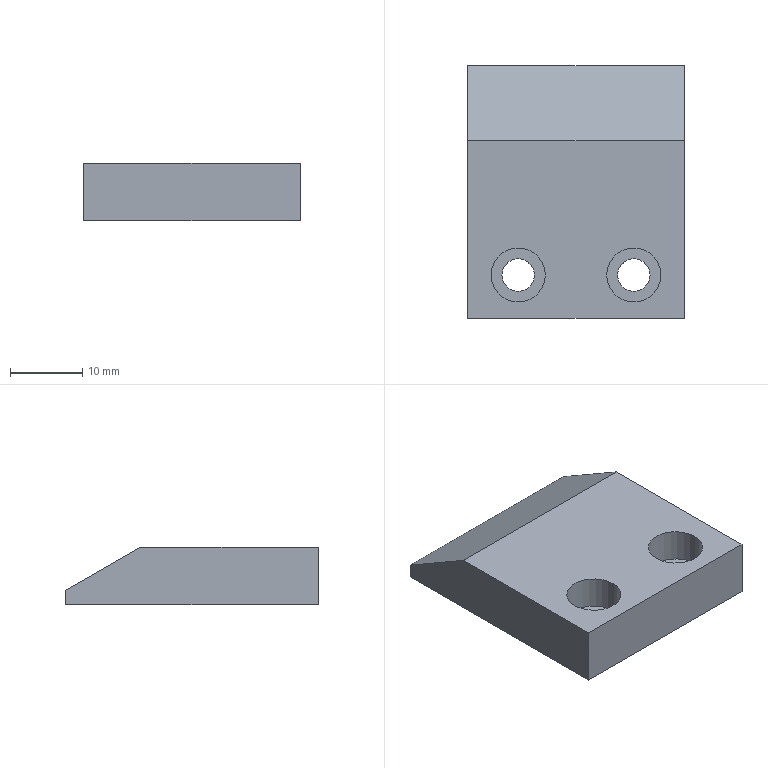Part | STEP file | BPSP-03-015 Shaft Pivot Seat | 1 solid | 17 faces | box 30 x 35 x 8 mm | volume 6950 mm3 | plane 9 | cylinder 8 | commonest cylinder face diameters 4.5 x4 7.5 x4
STEP:
#1=CARTESIAN_POINT('',(0.,0.,0.));
#2=DIRECTION('',(0.,0.,1.));
#3=DIRECTION('',(1.,0.,0.));
#4=AXIS2_PLACEMENT_3D('',#1,#2,#3);
#5=CARTESIAN_POINT('',(11.75,0.,-0.6));
#6=VERTEX_POINT('',#5);
#7=CARTESIAN_POINT('',(11.75,0.,4.));
#8=VERTEX_POINT('',#7);
#9=CARTESIAN_POINT('',(11.75,0.,4.));
#10=DIRECTION('',(0.,0.,1.));
#11=VECTOR('',#10,1.);
#12=LINE('',#9,#11);
#13=CARTESIAN_POINT('',(8.,0.,4.));
#14=DIRECTION('',(0.,0.,1.));
#15=DIRECTION('',(1.,0.,0.));
#16=AXIS2_PLACEMENT_3D('',#13,#14,#15);
#17=CYLINDRICAL_SURFACE('',#16,3.75);
#18=CARTESIAN_POINT('',(6.283,0.));
#19=DIRECTION('',(0.,1.));
#20=VECTOR('',#19,1.);
#21=LINE('',#18,#20);
#22=(GEOMETRIC_REPRESENTATION_CONTEXT(2)PARAMETRIC_REPRESENTATION_CONTEXT()REPRESENTATION_CONTEXT('',''));
#23=DEFINITIONAL_REPRESENTATION('',(#21),#22);
#24=PCURVE('',#17,#23);
#25=CARTESIAN_POINT('',(8.,0.,4.));
#26=DIRECTION('',(0.,0.,1.));
#27=DIRECTION('',(1.,0.,0.));
#28=AXIS2_PLACEMENT_3D('',#25,#26,#27);
#29=CYLINDRICAL_SURFACE('',#28,3.75);
#30=CARTESIAN_POINT('',(0.,0.));
#31=DIRECTION('',(0.,1.));
#32=VECTOR('',#31,1.);
#33=LINE('',#30,#32);
#34=(GEOMETRIC_REPRESENTATION_CONTEXT(2)PARAMETRIC_REPRESENTATION_CONTEXT()REPRESENTATION_CONTEXT('',''));
#35=DEFINITIONAL_REPRESENTATION('',(#33),#34);
#36=PCURVE('',#29,#35);
#37=SURFACE_CURVE('',#12,(#24,#36),.PCURVE_S1.);
#38=EDGE_CURVE('',#6,#8,#37,.T.);
#39=ORIENTED_EDGE('',*,*,#38,.T.);
#40=CARTESIAN_POINT('',(4.25,0.,4.));
#41=VERTEX_POINT('',#40);
#42=CARTESIAN_POINT('',(8.,0.,4.));
#43=DIRECTION('',(0.,0.,1.));
#44=DIRECTION('',(1.,0.,0.));
#45=AXIS2_PLACEMENT_3D('',#42,#43,#44);
#46=CIRCLE('',#45,3.75);
#47=CARTESIAN_POINT('',(0.,0.));
#48=DIRECTION('',(1.,0.));
#49=VECTOR('',#48,1.);
#50=LINE('',#47,#49);
#51=(GEOMETRIC_REPRESENTATION_CONTEXT(2)PARAMETRIC_REPRESENTATION_CONTEXT()REPRESENTATION_CONTEXT('',''));
#52=DEFINITIONAL_REPRESENTATION('',(#50),#51);
#53=PCURVE('',#17,#52);
#54=CARTESIAN_POINT('',(0.,0.,4.));
#55=DIRECTION('',(0.,0.,1.));
#56=DIRECTION('',(1.,0.,0.));
#57=AXIS2_PLACEMENT_3D('',#54,#55,#56);
#58=PLANE('',#57);
#59=CARTESIAN_POINT('',(8.,0.));
#60=DIRECTION('',(1.,0.));
#61=AXIS2_PLACEMENT_2D('',#59,#60);
#62=CIRCLE('',#61,3.75);
#63=(GEOMETRIC_REPRESENTATION_CONTEXT(2)PARAMETRIC_REPRESENTATION_CONTEXT()REPRESENTATION_CONTEXT('',''));
#64=DEFINITIONAL_REPRESENTATION('',(#62),#63);
#65=PCURVE('',#58,#64);
#66=SURFACE_CURVE('',#46,(#53,#65),.PCURVE_S1.);
#67=EDGE_CURVE('',#41,#8,#66,.T.);
#68=ORIENTED_EDGE('',*,*,#67,.F.);
#69=CARTESIAN_POINT('',(4.25,0.,-0.6));
#70=VERTEX_POINT('',#69);
#71=CARTESIAN_POINT('',(4.25,0.,4.));
#72=DIRECTION('',(0.,0.,1.));
#73=VECTOR('',#72,1.);
#74=LINE('',#71,#73);
#75=CARTESIAN_POINT('',(3.142,0.));
#76=DIRECTION('',(0.,1.));
#77=VECTOR('',#76,1.);
#78=LINE('',#75,#77);
#79=(GEOMETRIC_REPRESENTATION_CONTEXT(2)PARAMETRIC_REPRESENTATION_CONTEXT()REPRESENTATION_CONTEXT('',''));
#80=DEFINITIONAL_REPRESENTATION('',(#78),#79);
#81=PCURVE('',#17,#80);
#82=CARTESIAN_POINT('',(3.142,0.));
#83=DIRECTION('',(0.,1.));
#84=VECTOR('',#83,1.);
#85=LINE('',#82,#84);
#86=(GEOMETRIC_REPRESENTATION_CONTEXT(2)PARAMETRIC_REPRESENTATION_CONTEXT()REPRESENTATION_CONTEXT('',''));
#87=DEFINITIONAL_REPRESENTATION('',(#85),#86);
#88=PCURVE('',#29,#87);
#89=SURFACE_CURVE('',#74,(#81,#88),.PCURVE_S1.);
#90=EDGE_CURVE('',#70,#41,#89,.T.);
#91=ORIENTED_EDGE('',*,*,#90,.F.);
#92=CARTESIAN_POINT('',(8.,0.,-0.6));
#93=DIRECTION('',(0.,0.,1.));
#94=DIRECTION('',(1.,0.,0.));
#95=AXIS2_PLACEMENT_3D('',#92,#93,#94);
#96=CIRCLE('',#95,3.75);
#97=CARTESIAN_POINT('',(0.,-4.6));
#98=DIRECTION('',(1.,0.));
#99=VECTOR('',#98,1.);
#100=LINE('',#97,#99);
#101=(GEOMETRIC_REPRESENTATION_CONTEXT(2)PARAMETRIC_REPRESENTATION_CONTEXT()REPRESENTATION_CONTEXT('',''));
#102=DEFINITIONAL_REPRESENTATION('',(#100),#101);
#103=PCURVE('',#17,#102);
#104=CARTESIAN_POINT('',(10.25,0.,-0.6));
#105=DIRECTION('',(0.,0.,-1.));
#106=DIRECTION('',(-1.,0.,0.));
#107=AXIS2_PLACEMENT_3D('',#104,#105,#106);
#108=PLANE('',#107);
#109=CARTESIAN_POINT('',(-1.5,0.));
#110=CARTESIAN_POINT('',(-1.5,6.495));
#111=CARTESIAN_POINT('',(4.125,3.248));
#112=CARTESIAN_POINT('',(9.75,0.));
#113=CARTESIAN_POINT('',(4.125,-3.248));
#114=CARTESIAN_POINT('',(-1.5,-6.495));
#115=CARTESIAN_POINT('',(-1.5,0.));
#116=(BOUNDED_CURVE()B_SPLINE_CURVE(2,(#109,#110,#111,#112,#113,#114,#115),.UNSPECIFIED.,.T.,.F.)B_SPLINE_CURVE_WITH_KNOTS((1,2,2,2,2,1),(-2.094,0.,2.094,4.189,6.283,8.378),.UNSPECIFIED.)CURVE()GEOMETRIC_REPRESENTATION_ITEM()RATIONAL_B_SPLINE_CURVE((1.,0.5,1.,0.5,1.,0.5,1.))REPRESENTATION_ITEM(''));
#117=(GEOMETRIC_REPRESENTATION_CONTEXT(2)PARAMETRIC_REPRESENTATION_CONTEXT()REPRESENTATION_CONTEXT('',''));
#118=DEFINITIONAL_REPRESENTATION('',(#116),#117);
#119=PCURVE('',#108,#118);
#120=SURFACE_CURVE('',#96,(#103,#119),.PCURVE_S1.);
#121=EDGE_CURVE('',#70,#6,#120,.T.);
#122=ORIENTED_EDGE('',*,*,#121,.T.);
#123=EDGE_LOOP('',(#39,#68,#91,#122));
#124=FACE_BOUND('',#123,.F.);
#125=ADVANCED_FACE('',(#124),#17,.F.);
#126=CARTESIAN_POINT('',(10.25,0.,-4.));
#127=VERTEX_POINT('',#126);
#128=CARTESIAN_POINT('',(10.25,0.,-0.6));
#129=VERTEX_POINT('',#128);
#130=CARTESIAN_POINT('',(10.25,0.,4.));
#131=DIRECTION('',(0.,0.,1.));
#132=VECTOR('',#131,1.);
#133=LINE('',#130,#132);
#134=CARTESIAN_POINT('',(8.,0.,4.));
#135=DIRECTION('',(0.,0.,1.));
#136=DIRECTION('',(1.,0.,0.));
#137=AXIS2_PLACEMENT_3D('',#134,#135,#136);
#138=CYLINDRICAL_SURFACE('',#137,2.25);
#139=CARTESIAN_POINT('',(6.283,0.));
#140=DIRECTION('',(0.,1.));
#141=VECTOR('',#140,1.);
#142=LINE('',#139,#141);
#143=(GEOMETRIC_REPRESENTATION_CONTEXT(2)PARAMETRIC_REPRESENTATION_CONTEXT()REPRESENTATION_CONTEXT('',''));
#144=DEFINITIONAL_REPRESENTATION('',(#142),#143);
#145=PCURVE('',#138,#144);
#146=CARTESIAN_POINT('',(8.,0.,4.));
#147=DIRECTION('',(0.,0.,1.));
#148=DIRECTION('',(1.,0.,0.));
#149=AXIS2_PLACEMENT_3D('',#146,#147,#148);
#150=CYLINDRICAL_SURFACE('',#149,2.25);
#151=CARTESIAN_POINT('',(0.,0.));
#152=DIRECTION('',(0.,1.));
#153=VECTOR('',#152,1.);
#154=LINE('',#151,#153);
#155=(GEOMETRIC_REPRESENTATION_CONTEXT(2)PARAMETRIC_REPRESENTATION_CONTEXT()REPRESENTATION_CONTEXT('',''));
#156=DEFINITIONAL_REPRESENTATION('',(#154),#155);
#157=PCURVE('',#150,#156);
#158=SURFACE_CURVE('',#133,(#145,#157),.PCURVE_S1.);
#159=EDGE_CURVE('',#127,#129,#158,.T.);
#160=ORIENTED_EDGE('',*,*,#159,.T.);
#161=CARTESIAN_POINT('',(5.75,0.,-0.6));
#162=VERTEX_POINT('',#161);
#163=CARTESIAN_POINT('',(8.,0.,-0.6));
#164=DIRECTION('',(0.,0.,1.));
#165=DIRECTION('',(1.,0.,0.));
#166=AXIS2_PLACEMENT_3D('',#163,#164,#165);
#167=CIRCLE('',#166,2.25);
#168=CARTESIAN_POINT('',(0.,-4.6));
#169=DIRECTION('',(1.,0.));
#170=VECTOR('',#169,1.);
#171=LINE('',#168,#170);
#172=(GEOMETRIC_REPRESENTATION_CONTEXT(2)PARAMETRIC_REPRESENTATION_CONTEXT()REPRESENTATION_CONTEXT('',''));
#173=DEFINITIONAL_REPRESENTATION('',(#171),#172);
#174=PCURVE('',#138,#173);
#175=CARTESIAN_POINT('',(0.,0.));
#176=CARTESIAN_POINT('',(0.,3.897));
#177=CARTESIAN_POINT('',(3.375,1.949));
#178=CARTESIAN_POINT('',(6.75,0.));
#179=CARTESIAN_POINT('',(3.375,-1.949));
#180=CARTESIAN_POINT('',(0.,-3.897));
#181=CARTESIAN_POINT('',(0.,0.));
#182=(BOUNDED_CURVE()B_SPLINE_CURVE(2,(#175,#176,#177,#178,#179,#180,#181),.UNSPECIFIED.,.T.,.F.)B_SPLINE_CURVE_WITH_KNOTS((1,2,2,2,2,1),(-2.094,0.,2.094,4.189,6.283,8.378),.UNSPECIFIED.)CURVE()GEOMETRIC_REPRESENTATION_ITEM()RATIONAL_B_SPLINE_CURVE((1.,0.5,1.,0.5,1.,0.5,1.))REPRESENTATION_ITEM(''));
#183=(GEOMETRIC_REPRESENTATION_CONTEXT(2)PARAMETRIC_REPRESENTATION_CONTEXT()REPRESENTATION_CONTEXT('',''));
#184=DEFINITIONAL_REPRESENTATION('',(#182),#183);
#185=PCURVE('',#108,#184);
#186=SURFACE_CURVE('',#167,(#174,#185),.PCURVE_S1.);
#187=EDGE_CURVE('',#162,#129,#186,.T.);
#188=ORIENTED_EDGE('',*,*,#187,.F.);
#189=CARTESIAN_POINT('',(5.75,0.,-4.));
#190=VERTEX_POINT('',#189);
#191=CARTESIAN_POINT('',(5.75,0.,4.));
#192=DIRECTION('',(0.,0.,1.));
#193=VECTOR('',#192,1.);
#194=LINE('',#191,#193);
#195=CARTESIAN_POINT('',(3.142,0.));
#196=DIRECTION('',(0.,1.));
#197=VECTOR('',#196,1.);
#198=LINE('',#195,#197);
#199=(GEOMETRIC_REPRESENTATION_CONTEXT(2)PARAMETRIC_REPRESENTATION_CONTEXT()REPRESENTATION_CONTEXT('',''));
#200=DEFINITIONAL_REPRESENTATION('',(#198),#199);
#201=PCURVE('',#138,#200);
#202=CARTESIAN_POINT('',(3.142,0.));
#203=DIRECTION('',(0.,1.));
#204=VECTOR('',#203,1.);
#205=LINE('',#202,#204);
#206=(GEOMETRIC_REPRESENTATION_CONTEXT(2)PARAMETRIC_REPRESENTATION_CONTEXT()REPRESENTATION_CONTEXT('',''));
#207=DEFINITIONAL_REPRESENTATION('',(#205),#206);
#208=PCURVE('',#150,#207);
#209=SURFACE_CURVE('',#194,(#201,#208),.PCURVE_S1.);
#210=EDGE_CURVE('',#190,#162,#209,.T.);
#211=ORIENTED_EDGE('',*,*,#210,.F.);
#212=CARTESIAN_POINT('',(8.,0.,-4.));
#213=DIRECTION('',(0.,0.,1.));
#214=DIRECTION('',(1.,0.,0.));
#215=AXIS2_PLACEMENT_3D('',#212,#213,#214);
#216=CIRCLE('',#215,2.25);
#217=CARTESIAN_POINT('',(0.,-8.));
#218=DIRECTION('',(1.,0.));
#219=VECTOR('',#218,1.);
#220=LINE('',#217,#219);
#221=(GEOMETRIC_REPRESENTATION_CONTEXT(2)PARAMETRIC_REPRESENTATION_CONTEXT()REPRESENTATION_CONTEXT('',''));
#222=DEFINITIONAL_REPRESENTATION('',(#220),#221);
#223=PCURVE('',#138,#222);
#224=CARTESIAN_POINT('',(0.,0.,-4.));
#225=DIRECTION('',(0.,0.,1.));
#226=DIRECTION('',(1.,0.,0.));
#227=AXIS2_PLACEMENT_3D('',#224,#225,#226);
#228=PLANE('',#227);
#229=CARTESIAN_POINT('',(8.,0.));
#230=DIRECTION('',(1.,0.));
#231=AXIS2_PLACEMENT_2D('',#229,#230);
#232=CIRCLE('',#231,2.25);
#233=(GEOMETRIC_REPRESENTATION_CONTEXT(2)PARAMETRIC_REPRESENTATION_CONTEXT()REPRESENTATION_CONTEXT('',''));
#234=DEFINITIONAL_REPRESENTATION('',(#232),#233);
#235=PCURVE('',#228,#234);
#236=SURFACE_CURVE('',#216,(#223,#235),.PCURVE_S1.);
#237=EDGE_CURVE('',#190,#127,#236,.T.);
#238=ORIENTED_EDGE('',*,*,#237,.T.);
#239=EDGE_LOOP('',(#160,#188,#211,#238));
#240=FACE_BOUND('',#239,.F.);
#241=ADVANCED_FACE('',(#240),#138,.F.);
#242=CARTESIAN_POINT('',(-4.25,0.,-0.6));
#243=VERTEX_POINT('',#242);
#244=CARTESIAN_POINT('',(-4.25,0.,4.));
#245=VERTEX_POINT('',#244);
#246=CARTESIAN_POINT('',(-4.25,0.,4.));
#247=DIRECTION('',(0.,0.,1.));
#248=VECTOR('',#247,1.);
#249=LINE('',#246,#248);
#250=CARTESIAN_POINT('',(-8.,0.,4.));
#251=DIRECTION('',(0.,0.,1.));
#252=DIRECTION('',(1.,0.,0.));
#253=AXIS2_PLACEMENT_3D('',#250,#251,#252);
#254=CYLINDRICAL_SURFACE('',#253,3.75);
#255=CARTESIAN_POINT('',(6.283,0.));
#256=DIRECTION('',(0.,1.));
#257=VECTOR('',#256,1.);
#258=LINE('',#255,#257);
#259=(GEOMETRIC_REPRESENTATION_CONTEXT(2)PARAMETRIC_REPRESENTATION_CONTEXT()REPRESENTATION_CONTEXT('',''));
#260=DEFINITIONAL_REPRESENTATION('',(#258),#259);
#261=PCURVE('',#254,#260);
#262=CARTESIAN_POINT('',(-8.,0.,4.));
#263=DIRECTION('',(0.,0.,1.));
#264=DIRECTION('',(1.,0.,0.));
#265=AXIS2_PLACEMENT_3D('',#262,#263,#264);
#266=CYLINDRICAL_SURFACE('',#265,3.75);
#267=CARTESIAN_POINT('',(0.,0.));
#268=DIRECTION('',(0.,1.));
#269=VECTOR('',#268,1.);
#270=LINE('',#267,#269);
#271=(GEOMETRIC_REPRESENTATION_CONTEXT(2)PARAMETRIC_REPRESENTATION_CONTEXT()REPRESENTATION_CONTEXT('',''));
#272=DEFINITIONAL_REPRESENTATION('',(#270),#271);
#273=PCURVE('',#266,#272);
#274=SURFACE_CURVE('',#249,(#261,#273),.PCURVE_S1.);
#275=EDGE_CURVE('',#243,#245,#274,.T.);
#276=ORIENTED_EDGE('',*,*,#275,.T.);
#277=CARTESIAN_POINT('',(-11.75,0.,4.));
#278=VERTEX_POINT('',#277);
#279=CARTESIAN_POINT('',(-8.,0.,4.));
#280=DIRECTION('',(0.,0.,1.));
#281=DIRECTION('',(1.,0.,0.));
#282=AXIS2_PLACEMENT_3D('',#279,#280,#281);
#283=CIRCLE('',#282,3.75);
#284=CARTESIAN_POINT('',(0.,0.));
#285=DIRECTION('',(1.,0.));
#286=VECTOR('',#285,1.);
#287=LINE('',#284,#286);
#288=(GEOMETRIC_REPRESENTATION_CONTEXT(2)PARAMETRIC_REPRESENTATION_CONTEXT()REPRESENTATION_CONTEXT('',''));
#289=DEFINITIONAL_REPRESENTATION('',(#287),#288);
#290=PCURVE('',#254,#289);
#291=CARTESIAN_POINT('',(-8.,0.));
#292=DIRECTION('',(1.,0.));
#293=AXIS2_PLACEMENT_2D('',#291,#292);
#294=CIRCLE('',#293,3.75);
#295=(GEOMETRIC_REPRESENTATION_CONTEXT(2)PARAMETRIC_REPRESENTATION_CONTEXT()REPRESENTATION_CONTEXT('',''));
#296=DEFINITIONAL_REPRESENTATION('',(#294),#295);
#297=PCURVE('',#58,#296);
#298=SURFACE_CURVE('',#283,(#290,#297),.PCURVE_S1.);
#299=EDGE_CURVE('',#278,#245,#298,.T.);
#300=ORIENTED_EDGE('',*,*,#299,.F.);
#301=CARTESIAN_POINT('',(-11.75,0.,-0.6));
#302=VERTEX_POINT('',#301);
#303=CARTESIAN_POINT('',(-11.75,0.,4.));
#304=DIRECTION('',(0.,0.,1.));
#305=VECTOR('',#304,1.);
#306=LINE('',#303,#305);
#307=CARTESIAN_POINT('',(3.142,0.));
#308=DIRECTION('',(0.,1.));
#309=VECTOR('',#308,1.);
#310=LINE('',#307,#309);
#311=(GEOMETRIC_REPRESENTATION_CONTEXT(2)PARAMETRIC_REPRESENTATION_CONTEXT()REPRESENTATION_CONTEXT('',''));
#312=DEFINITIONAL_REPRESENTATION('',(#310),#311);
#313=PCURVE('',#254,#312);
#314=CARTESIAN_POINT('',(3.142,0.));
#315=DIRECTION('',(0.,1.));
#316=VECTOR('',#315,1.);
#317=LINE('',#314,#316);
#318=(GEOMETRIC_REPRESENTATION_CONTEXT(2)PARAMETRIC_REPRESENTATION_CONTEXT()REPRESENTATION_CONTEXT('',''));
#319=DEFINITIONAL_REPRESENTATION('',(#317),#318);
#320=PCURVE('',#266,#319);
#321=SURFACE_CURVE('',#306,(#313,#320),.PCURVE_S1.);
#322=EDGE_CURVE('',#302,#278,#321,.T.);
#323=ORIENTED_EDGE('',*,*,#322,.F.);
#324=CARTESIAN_POINT('',(-8.,0.,-0.6));
#325=DIRECTION('',(0.,0.,1.));
#326=DIRECTION('',(1.,0.,0.));
#327=AXIS2_PLACEMENT_3D('',#324,#325,#326);
#328=CIRCLE('',#327,3.75);
#329=CARTESIAN_POINT('',(0.,-4.6));
#330=DIRECTION('',(1.,0.));
#331=VECTOR('',#330,1.);
#332=LINE('',#329,#331);
#333=(GEOMETRIC_REPRESENTATION_CONTEXT(2)PARAMETRIC_REPRESENTATION_CONTEXT()REPRESENTATION_CONTEXT('',''));
#334=DEFINITIONAL_REPRESENTATION('',(#332),#333);
#335=PCURVE('',#254,#334);
#336=CARTESIAN_POINT('',(-5.75,0.,-0.6));
#337=DIRECTION('',(0.,0.,-1.));
#338=DIRECTION('',(-1.,0.,0.));
#339=AXIS2_PLACEMENT_3D('',#336,#337,#338);
#340=PLANE('',#339);
#341=CARTESIAN_POINT('',(-1.5,0.));
#342=CARTESIAN_POINT('',(-1.5,6.495));
#343=CARTESIAN_POINT('',(4.125,3.248));
#344=CARTESIAN_POINT('',(9.75,0.));
#345=CARTESIAN_POINT('',(4.125,-3.248));
#346=CARTESIAN_POINT('',(-1.5,-6.495));
#347=CARTESIAN_POINT('',(-1.5,0.));
#348=(BOUNDED_CURVE()B_SPLINE_CURVE(2,(#341,#342,#343,#344,#345,#346,#347),.UNSPECIFIED.,.T.,.F.)B_SPLINE_CURVE_WITH_KNOTS((1,2,2,2,2,1),(-2.094,0.,2.094,4.189,6.283,8.378),.UNSPECIFIED.)CURVE()GEOMETRIC_REPRESENTATION_ITEM()RATIONAL_B_SPLINE_CURVE((1.,0.5,1.,0.5,1.,0.5,1.))REPRESENTATION_ITEM(''));
#349=(GEOMETRIC_REPRESENTATION_CONTEXT(2)PARAMETRIC_REPRESENTATION_CONTEXT()REPRESENTATION_CONTEXT('',''));
#350=DEFINITIONAL_REPRESENTATION('',(#348),#349);
#351=PCURVE('',#340,#350);
#352=SURFACE_CURVE('',#328,(#335,#351),.PCURVE_S1.);
#353=EDGE_CURVE('',#302,#243,#352,.T.);
#354=ORIENTED_EDGE('',*,*,#353,.T.);
#355=EDGE_LOOP('',(#276,#300,#323,#354));
#356=FACE_BOUND('',#355,.F.);
#357=ADVANCED_FACE('',(#356),#254,.F.);
#358=CARTESIAN_POINT('',(-5.75,0.,-4.));
#359=VERTEX_POINT('',#358);
#360=CARTESIAN_POINT('',(-5.75,0.,-0.6));
#361=VERTEX_POINT('',#360);
#362=CARTESIAN_POINT('',(-5.75,0.,4.));
#363=DIRECTION('',(0.,0.,1.));
#364=VECTOR('',#363,1.);
#365=LINE('',#362,#364);
#366=CARTESIAN_POINT('',(-8.,0.,4.));
#367=DIRECTION('',(0.,0.,1.));
#368=DIRECTION('',(1.,0.,0.));
#369=AXIS2_PLACEMENT_3D('',#366,#367,#368);
#370=CYLINDRICAL_SURFACE('',#369,2.25);
#371=CARTESIAN_POINT('',(6.283,0.));
#372=DIRECTION('',(0.,1.));
#373=VECTOR('',#372,1.);
#374=LINE('',#371,#373);
#375=(GEOMETRIC_REPRESENTATION_CONTEXT(2)PARAMETRIC_REPRESENTATION_CONTEXT()REPRESENTATION_CONTEXT('',''));
#376=DEFINITIONAL_REPRESENTATION('',(#374),#375);
#377=PCURVE('',#370,#376);
#378=CARTESIAN_POINT('',(-8.,0.,4.));
#379=DIRECTION('',(0.,0.,1.));
#380=DIRECTION('',(1.,0.,0.));
#381=AXIS2_PLACEMENT_3D('',#378,#379,#380);
#382=CYLINDRICAL_SURFACE('',#381,2.25);
#383=CARTESIAN_POINT('',(0.,0.));
#384=DIRECTION('',(0.,1.));
#385=VECTOR('',#384,1.);
#386=LINE('',#383,#385);
#387=(GEOMETRIC_REPRESENTATION_CONTEXT(2)PARAMETRIC_REPRESENTATION_CONTEXT()REPRESENTATION_CONTEXT('',''));
#388=DEFINITIONAL_REPRESENTATION('',(#386),#387);
#389=PCURVE('',#382,#388);
#390=SURFACE_CURVE('',#365,(#377,#389),.PCURVE_S1.);
#391=EDGE_CURVE('',#359,#361,#390,.T.);
#392=ORIENTED_EDGE('',*,*,#391,.T.);
#393=CARTESIAN_POINT('',(-10.25,0.,-0.6));
#394=VERTEX_POINT('',#393);
#395=CARTESIAN_POINT('',(-8.,0.,-0.6));
#396=DIRECTION('',(0.,0.,1.));
#397=DIRECTION('',(1.,0.,0.));
#398=AXIS2_PLACEMENT_3D('',#395,#396,#397);
#399=CIRCLE('',#398,2.25);
#400=CARTESIAN_POINT('',(0.,-4.6));
#401=DIRECTION('',(1.,0.));
#402=VECTOR('',#401,1.);
#403=LINE('',#400,#402);
#404=(GEOMETRIC_REPRESENTATION_CONTEXT(2)PARAMETRIC_REPRESENTATION_CONTEXT()REPRESENTATION_CONTEXT('',''));
#405=DEFINITIONAL_REPRESENTATION('',(#403),#404);
#406=PCURVE('',#370,#405);
#407=CARTESIAN_POINT('',(0.,0.));
#408=CARTESIAN_POINT('',(0.,3.897));
#409=CARTESIAN_POINT('',(3.375,1.949));
#410=CARTESIAN_POINT('',(6.75,0.));
#411=CARTESIAN_POINT('',(3.375,-1.949));
#412=CARTESIAN_POINT('',(0.,-3.897));
#413=CARTESIAN_POINT('',(0.,0.));
#414=(BOUNDED_CURVE()B_SPLINE_CURVE(2,(#407,#408,#409,#410,#411,#412,#413),.UNSPECIFIED.,.T.,.F.)B_SPLINE_CURVE_WITH_KNOTS((1,2,2,2,2,1),(-2.094,0.,2.094,4.189,6.283,8.378),.UNSPECIFIED.)CURVE()GEOMETRIC_REPRESENTATION_ITEM()RATIONAL_B_SPLINE_CURVE((1.,0.5,1.,0.5,1.,0.5,1.))REPRESENTATION_ITEM(''));
#415=(GEOMETRIC_REPRESENTATION_CONTEXT(2)PARAMETRIC_REPRESENTATION_CONTEXT()REPRESENTATION_CONTEXT('',''));
#416=DEFINITIONAL_REPRESENTATION('',(#414),#415);
#417=PCURVE('',#340,#416);
#418=SURFACE_CURVE('',#399,(#406,#417),.PCURVE_S1.);
#419=EDGE_CURVE('',#394,#361,#418,.T.);
#420=ORIENTED_EDGE('',*,*,#419,.F.);
#421=CARTESIAN_POINT('',(-10.25,0.,-4.));
#422=VERTEX_POINT('',#421);
#423=CARTESIAN_POINT('',(-10.25,0.,4.));
#424=DIRECTION('',(0.,0.,1.));
#425=VECTOR('',#424,1.);
#426=LINE('',#423,#425);
#427=CARTESIAN_POINT('',(3.142,0.));
#428=DIRECTION('',(0.,1.));
#429=VECTOR('',#428,1.);
#430=LINE('',#427,#429);
#431=(GEOMETRIC_REPRESENTATION_CONTEXT(2)PARAMETRIC_REPRESENTATION_CONTEXT()REPRESENTATION_CONTEXT('',''));
#432=DEFINITIONAL_REPRESENTATION('',(#430),#431);
#433=PCURVE('',#370,#432);
#434=CARTESIAN_POINT('',(3.142,0.));
#435=DIRECTION('',(0.,1.));
#436=VECTOR('',#435,1.);
#437=LINE('',#434,#436);
#438=(GEOMETRIC_REPRESENTATION_CONTEXT(2)PARAMETRIC_REPRESENTATION_CONTEXT()REPRESENTATION_CONTEXT('',''));
#439=DEFINITIONAL_REPRESENTATION('',(#437),#438);
#440=PCURVE('',#382,#439);
#441=SURFACE_CURVE('',#426,(#433,#440),.PCURVE_S1.);
#442=EDGE_CURVE('',#422,#394,#441,.T.);
#443=ORIENTED_EDGE('',*,*,#442,.F.);
#444=CARTESIAN_POINT('',(-8.,0.,-4.));
#445=DIRECTION('',(0.,0.,1.));
#446=DIRECTION('',(1.,0.,0.));
#447=AXIS2_PLACEMENT_3D('',#444,#445,#446);
#448=CIRCLE('',#447,2.25);
#449=CARTESIAN_POINT('',(0.,-8.));
#450=DIRECTION('',(1.,0.));
#451=VECTOR('',#450,1.);
#452=LINE('',#449,#451);
#453=(GEOMETRIC_REPRESENTATION_CONTEXT(2)PARAMETRIC_REPRESENTATION_CONTEXT()REPRESENTATION_CONTEXT('',''));
#454=DEFINITIONAL_REPRESENTATION('',(#452),#453);
#455=PCURVE('',#370,#454);
#456=CARTESIAN_POINT('',(-8.,0.));
#457=DIRECTION('',(1.,0.));
#458=AXIS2_PLACEMENT_2D('',#456,#457);
#459=CIRCLE('',#458,2.25);
#460=(GEOMETRIC_REPRESENTATION_CONTEXT(2)PARAMETRIC_REPRESENTATION_CONTEXT()REPRESENTATION_CONTEXT('',''));
#461=DEFINITIONAL_REPRESENTATION('',(#459),#460);
#462=PCURVE('',#228,#461);
#463=SURFACE_CURVE('',#448,(#455,#462),.PCURVE_S1.);
#464=EDGE_CURVE('',#422,#359,#463,.T.);
#465=ORIENTED_EDGE('',*,*,#464,.T.);
#466=EDGE_LOOP('',(#392,#420,#443,#465));
#467=FACE_BOUND('',#466,.F.);
#468=ADVANCED_FACE('',(#467),#370,.F.);
#469=CARTESIAN_POINT('',(-15.,18.608,4.));
#470=VERTEX_POINT('',#469);
#471=CARTESIAN_POINT('',(-15.,-6.,4.));
#472=VERTEX_POINT('',#471);
#473=CARTESIAN_POINT('',(-15.,29.,4.));
#474=DIRECTION('',(0.,-1.,0.));
#475=VECTOR('',#474,1.);
#476=LINE('',#473,#475);
#477=CARTESIAN_POINT('',(-15.,29.,4.));
#478=DIRECTION('',(1.,0.,0.));
#479=DIRECTION('',(0.,1.,0.));
#480=AXIS2_PLACEMENT_3D('',#477,#478,#479);
#481=PLANE('',#480);
#482=CARTESIAN_POINT('',(0.,0.));
#483=DIRECTION('',(-1.,0.));
#484=VECTOR('',#483,1.);
#485=LINE('',#482,#484);
#486=(GEOMETRIC_REPRESENTATION_CONTEXT(2)PARAMETRIC_REPRESENTATION_CONTEXT()REPRESENTATION_CONTEXT('',''));
#487=DEFINITIONAL_REPRESENTATION('',(#485),#486);
#488=PCURVE('',#481,#487);
#489=CARTESIAN_POINT('',(-15.,29.));
#490=DIRECTION('',(0.,-1.));
#491=VECTOR('',#490,1.);
#492=LINE('',#489,#491);
#493=(GEOMETRIC_REPRESENTATION_CONTEXT(2)PARAMETRIC_REPRESENTATION_CONTEXT()REPRESENTATION_CONTEXT('',''));
#494=DEFINITIONAL_REPRESENTATION('',(#492),#493);
#495=PCURVE('',#58,#494);
#496=SURFACE_CURVE('',#476,(#488,#495),.PCURVE_S1.);
#497=EDGE_CURVE('',#470,#472,#496,.T.);
#498=ORIENTED_EDGE('',*,*,#497,.F.);
#499=CARTESIAN_POINT('',(-15.,29.,-2.));
#500=VERTEX_POINT('',#499);
#501=CARTESIAN_POINT('',(-15.,18.608,4.));
#502=DIRECTION('',(0.,0.866,-0.5));
#503=VECTOR('',#502,1.);
#504=LINE('',#501,#503);
#505=CARTESIAN_POINT('',(-10.392,0.));
#506=DIRECTION('',(0.866,-0.5));
#507=VECTOR('',#506,1.);
#508=LINE('',#505,#507);
#509=(GEOMETRIC_REPRESENTATION_CONTEXT(2)PARAMETRIC_REPRESENTATION_CONTEXT()REPRESENTATION_CONTEXT('',''));
#510=DEFINITIONAL_REPRESENTATION('',(#508),#509);
#511=PCURVE('',#481,#510);
#512=CARTESIAN_POINT('',(0.,18.608,4.));
#513=DIRECTION('',(0.,0.5,0.866));
#514=DIRECTION('',(1.,0.,0.));
#515=AXIS2_PLACEMENT_3D('',#512,#513,#514);
#516=PLANE('',#515);
#517=CARTESIAN_POINT('',(-15.,0.));
#518=DIRECTION('',(0.,1.));
#519=VECTOR('',#518,1.);
#520=LINE('',#517,#519);
#521=(GEOMETRIC_REPRESENTATION_CONTEXT(2)PARAMETRIC_REPRESENTATION_CONTEXT()REPRESENTATION_CONTEXT('',''));
#522=DEFINITIONAL_REPRESENTATION('',(#520),#521);
#523=PCURVE('',#516,#522);
#524=SURFACE_CURVE('',#504,(#511,#523),.PCURVE_S1.);
#525=EDGE_CURVE('',#470,#500,#524,.T.);
#526=ORIENTED_EDGE('',*,*,#525,.T.);
#527=CARTESIAN_POINT('',(-15.,29.,-4.));
#528=VERTEX_POINT('',#527);
#529=CARTESIAN_POINT('',(-15.,29.,4.));
#530=DIRECTION('',(0.,0.,-1.));
#531=VECTOR('',#530,1.);
#532=LINE('',#529,#531);
#533=CARTESIAN_POINT('',(0.,0.));
#534=DIRECTION('',(0.,-1.));
#535=VECTOR('',#534,1.);
#536=LINE('',#533,#535);
#537=(GEOMETRIC_REPRESENTATION_CONTEXT(2)PARAMETRIC_REPRESENTATION_CONTEXT()REPRESENTATION_CONTEXT('',''));
#538=DEFINITIONAL_REPRESENTATION('',(#536),#537);
#539=PCURVE('',#481,#538);
#540=CARTESIAN_POINT('',(-15.,29.,4.));
#541=DIRECTION('',(0.,-1.,0.));
#542=DIRECTION('',(1.,0.,0.));
#543=AXIS2_PLACEMENT_3D('',#540,#541,#542);
#544=PLANE('',#543);
#545=CARTESIAN_POINT('',(0.,0.));
#546=DIRECTION('',(0.,-1.));
#547=VECTOR('',#546,1.);
#548=LINE('',#545,#547);
#549=(GEOMETRIC_REPRESENTATION_CONTEXT(2)PARAMETRIC_REPRESENTATION_CONTEXT()REPRESENTATION_CONTEXT('',''));
#550=DEFINITIONAL_REPRESENTATION('',(#548),#549);
#551=PCURVE('',#544,#550);
#552=SURFACE_CURVE('',#532,(#539,#551),.PCURVE_S1.);
#553=EDGE_CURVE('',#500,#528,#552,.T.);
#554=ORIENTED_EDGE('',*,*,#553,.T.);
#555=CARTESIAN_POINT('',(-15.,-6.,-4.));
#556=VERTEX_POINT('',#555);
#557=CARTESIAN_POINT('',(-15.,29.,-4.));
#558=DIRECTION('',(0.,-1.,0.));
#559=VECTOR('',#558,1.);
#560=LINE('',#557,#559);
#561=CARTESIAN_POINT('',(0.,-8.));
#562=DIRECTION('',(-1.,0.));
#563=VECTOR('',#562,1.);
#564=LINE('',#561,#563);
#565=(GEOMETRIC_REPRESENTATION_CONTEXT(2)PARAMETRIC_REPRESENTATION_CONTEXT()REPRESENTATION_CONTEXT('',''));
#566=DEFINITIONAL_REPRESENTATION('',(#564),#565);
#567=PCURVE('',#481,#566);
#568=CARTESIAN_POINT('',(-15.,29.));
#569=DIRECTION('',(0.,-1.));
#570=VECTOR('',#569,1.);
#571=LINE('',#568,#570);
#572=(GEOMETRIC_REPRESENTATION_CONTEXT(2)PARAMETRIC_REPRESENTATION_CONTEXT()REPRESENTATION_CONTEXT('',''));
#573=DEFINITIONAL_REPRESENTATION('',(#571),#572);
#574=PCURVE('',#228,#573);
#575=SURFACE_CURVE('',#560,(#567,#574),.PCURVE_S1.);
#576=EDGE_CURVE('',#528,#556,#575,.T.);
#577=ORIENTED_EDGE('',*,*,#576,.T.);
#578=CARTESIAN_POINT('',(-15.,-6.,4.));
#579=DIRECTION('',(0.,0.,-1.));
#580=VECTOR('',#579,1.);
#581=LINE('',#578,#580);
#582=CARTESIAN_POINT('',(-35.,0.));
#583=DIRECTION('',(0.,-1.));
#584=VECTOR('',#583,1.);
#585=LINE('',#582,#584);
#586=(GEOMETRIC_REPRESENTATION_CONTEXT(2)PARAMETRIC_REPRESENTATION_CONTEXT()REPRESENTATION_CONTEXT('',''));
#587=DEFINITIONAL_REPRESENTATION('',(#585),#586);
#588=PCURVE('',#481,#587);
#589=CARTESIAN_POINT('',(-15.,-6.,4.));
#590=DIRECTION('',(0.,1.,0.));
#591=DIRECTION('',(-1.,0.,0.));
#592=AXIS2_PLACEMENT_3D('',#589,#590,#591);
#593=PLANE('',#592);
#594=CARTESIAN_POINT('',(0.,0.));
#595=DIRECTION('',(0.,-1.));
#596=VECTOR('',#595,1.);
#597=LINE('',#594,#596);
#598=(GEOMETRIC_REPRESENTATION_CONTEXT(2)PARAMETRIC_REPRESENTATION_CONTEXT()REPRESENTATION_CONTEXT('',''));
#599=DEFINITIONAL_REPRESENTATION('',(#597),#598);
#600=PCURVE('',#593,#599);
#601=SURFACE_CURVE('',#581,(#588,#600),.PCURVE_S1.);
#602=EDGE_CURVE('',#472,#556,#601,.T.);
#603=ORIENTED_EDGE('',*,*,#602,.F.);
#604=EDGE_LOOP('',(#498,#526,#554,#577,#603));
#605=FACE_BOUND('',#604,.T.);
#606=ADVANCED_FACE('',(#605),#481,.F.);
#607=CARTESIAN_POINT('',(15.,-6.,-4.));
#608=VERTEX_POINT('',#607);
#609=CARTESIAN_POINT('',(-15.,-6.,-4.));
#610=DIRECTION('',(1.,0.,0.));
#611=VECTOR('',#610,1.);
#612=LINE('',#609,#611);
#613=CARTESIAN_POINT('',(0.,-8.));
#614=DIRECTION('',(-1.,0.));
#615=VECTOR('',#614,1.);
#616=LINE('',#613,#615);
#617=(GEOMETRIC_REPRESENTATION_CONTEXT(2)PARAMETRIC_REPRESENTATION_CONTEXT()REPRESENTATION_CONTEXT('',''));
#618=DEFINITIONAL_REPRESENTATION('',(#616),#617);
#619=PCURVE('',#593,#618);
#620=CARTESIAN_POINT('',(-15.,-6.));
#621=DIRECTION('',(1.,0.));
#622=VECTOR('',#621,1.);
#623=LINE('',#620,#622);
#624=(GEOMETRIC_REPRESENTATION_CONTEXT(2)PARAMETRIC_REPRESENTATION_CONTEXT()REPRESENTATION_CONTEXT('',''));
#625=DEFINITIONAL_REPRESENTATION('',(#623),#624);
#626=PCURVE('',#228,#625);
#627=SURFACE_CURVE('',#612,(#619,#626),.PCURVE_S1.);
#628=EDGE_CURVE('',#556,#608,#627,.T.);
#629=ORIENTED_EDGE('',*,*,#628,.T.);
#630=CARTESIAN_POINT('',(15.,-6.,4.));
#631=VERTEX_POINT('',#630);
#632=CARTESIAN_POINT('',(15.,-6.,4.));
#633=DIRECTION('',(0.,0.,-1.));
#634=VECTOR('',#633,1.);
#635=LINE('',#632,#634);
#636=CARTESIAN_POINT('',(-30.,0.));
#637=DIRECTION('',(0.,-1.));
#638=VECTOR('',#637,1.);
#639=LINE('',#636,#638);
#640=(GEOMETRIC_REPRESENTATION_CONTEXT(2)PARAMETRIC_REPRESENTATION_CONTEXT()REPRESENTATION_CONTEXT('',''));
#641=DEFINITIONAL_REPRESENTATION('',(#639),#640);
#642=PCURVE('',#593,#641);
#643=CARTESIAN_POINT('',(15.,29.,4.));
#644=DIRECTION('',(-1.,0.,0.));
#645=DIRECTION('',(0.,0.,1.));
#646=AXIS2_PLACEMENT_3D('',#643,#644,#645);
#647=PLANE('',#646);
#648=CARTESIAN_POINT('',(0.,-35.));
#649=DIRECTION('',(-1.,0.));
#650=VECTOR('',#649,1.);
#651=LINE('',#648,#650);
#652=(GEOMETRIC_REPRESENTATION_CONTEXT(2)PARAMETRIC_REPRESENTATION_CONTEXT()REPRESENTATION_CONTEXT('',''));
#653=DEFINITIONAL_REPRESENTATION('',(#651),#652);
#654=PCURVE('',#647,#653);
#655=SURFACE_CURVE('',#635,(#642,#654),.PCURVE_S1.);
#656=EDGE_CURVE('',#631,#608,#655,.T.);
#657=ORIENTED_EDGE('',*,*,#656,.F.);
#658=CARTESIAN_POINT('',(-15.,-6.,4.));
#659=DIRECTION('',(1.,0.,0.));
#660=VECTOR('',#659,1.);
#661=LINE('',#658,#660);
#662=CARTESIAN_POINT('',(0.,0.));
#663=DIRECTION('',(-1.,0.));
#664=VECTOR('',#663,1.);
#665=LINE('',#662,#664);
#666=(GEOMETRIC_REPRESENTATION_CONTEXT(2)PARAMETRIC_REPRESENTATION_CONTEXT()REPRESENTATION_CONTEXT('',''));
#667=DEFINITIONAL_REPRESENTATION('',(#665),#666);
#668=PCURVE('',#593,#667);
#669=CARTESIAN_POINT('',(-15.,-6.));
#670=DIRECTION('',(1.,0.));
#671=VECTOR('',#670,1.);
#672=LINE('',#669,#671);
#673=(GEOMETRIC_REPRESENTATION_CONTEXT(2)PARAMETRIC_REPRESENTATION_CONTEXT()REPRESENTATION_CONTEXT('',''));
#674=DEFINITIONAL_REPRESENTATION('',(#672),#673);
#675=PCURVE('',#58,#674);
#676=SURFACE_CURVE('',#661,(#668,#675),.PCURVE_S1.);
#677=EDGE_CURVE('',#472,#631,#676,.T.);
#678=ORIENTED_EDGE('',*,*,#677,.F.);
#679=ORIENTED_EDGE('',*,*,#602,.T.);
#680=EDGE_LOOP('',(#629,#657,#678,#679));
#681=FACE_BOUND('',#680,.T.);
#682=ADVANCED_FACE('',(#681),#593,.F.);
#683=CARTESIAN_POINT('',(15.,29.,-2.));
#684=VERTEX_POINT('',#683);
#685=CARTESIAN_POINT('',(15.,29.,-4.));
#686=VERTEX_POINT('',#685);
#687=CARTESIAN_POINT('',(15.,29.,4.));
#688=DIRECTION('',(0.,0.,-1.));
#689=VECTOR('',#688,1.);
#690=LINE('',#687,#689);
#691=CARTESIAN_POINT('',(0.,0.));
#692=DIRECTION('',(-1.,0.));
#693=VECTOR('',#692,1.);
#694=LINE('',#691,#693);
#695=(GEOMETRIC_REPRESENTATION_CONTEXT(2)PARAMETRIC_REPRESENTATION_CONTEXT()REPRESENTATION_CONTEXT('',''));
#696=DEFINITIONAL_REPRESENTATION('',(#694),#695);
#697=PCURVE('',#647,#696);
#698=CARTESIAN_POINT('',(30.,0.));
#699=DIRECTION('',(0.,-1.));
#700=VECTOR('',#699,1.);
#701=LINE('',#698,#700);
#702=(GEOMETRIC_REPRESENTATION_CONTEXT(2)PARAMETRIC_REPRESENTATION_CONTEXT()REPRESENTATION_CONTEXT('',''));
#703=DEFINITIONAL_REPRESENTATION('',(#701),#702);
#704=PCURVE('',#544,#703);
#705=SURFACE_CURVE('',#690,(#697,#704),.PCURVE_S1.);
#706=EDGE_CURVE('',#684,#686,#705,.T.);
#707=ORIENTED_EDGE('',*,*,#706,.F.);
#708=CARTESIAN_POINT('',(15.,18.608,4.));
#709=VERTEX_POINT('',#708);
#710=CARTESIAN_POINT('',(15.,18.608,4.));
#711=DIRECTION('',(0.,-0.866,0.5));
#712=VECTOR('',#711,1.);
#713=LINE('',#710,#712);
#714=CARTESIAN_POINT('',(0.,-10.392));
#715=DIRECTION('',(0.5,-0.866));
#716=VECTOR('',#715,1.);
#717=LINE('',#714,#716);
#718=(GEOMETRIC_REPRESENTATION_CONTEXT(2)PARAMETRIC_REPRESENTATION_CONTEXT()REPRESENTATION_CONTEXT('',''));
#719=DEFINITIONAL_REPRESENTATION('',(#717),#718);
#720=PCURVE('',#647,#719);
#721=CARTESIAN_POINT('',(15.,0.));
#722=DIRECTION('',(0.,-1.));
#723=VECTOR('',#722,1.);
#724=LINE('',#721,#723);
#725=(GEOMETRIC_REPRESENTATION_CONTEXT(2)PARAMETRIC_REPRESENTATION_CONTEXT()REPRESENTATION_CONTEXT('',''));
#726=DEFINITIONAL_REPRESENTATION('',(#724),#725);
#727=PCURVE('',#516,#726);
#728=SURFACE_CURVE('',#713,(#720,#727),.PCURVE_S1.);
#729=EDGE_CURVE('',#684,#709,#728,.T.);
#730=ORIENTED_EDGE('',*,*,#729,.T.);
#731=CARTESIAN_POINT('',(15.,29.,4.));
#732=DIRECTION('',(0.,1.,0.));
#733=VECTOR('',#732,1.);
#734=LINE('',#731,#733);
#735=CARTESIAN_POINT('',(0.,0.));
#736=DIRECTION('',(0.,1.));
#737=VECTOR('',#736,1.);
#738=LINE('',#735,#737);
#739=(GEOMETRIC_REPRESENTATION_CONTEXT(2)PARAMETRIC_REPRESENTATION_CONTEXT()REPRESENTATION_CONTEXT('',''));
#740=DEFINITIONAL_REPRESENTATION('',(#738),#739);
#741=PCURVE('',#647,#740);
#742=CARTESIAN_POINT('',(15.,29.));
#743=DIRECTION('',(0.,1.));
#744=VECTOR('',#743,1.);
#745=LINE('',#742,#744);
#746=(GEOMETRIC_REPRESENTATION_CONTEXT(2)PARAMETRIC_REPRESENTATION_CONTEXT()REPRESENTATION_CONTEXT('',''));
#747=DEFINITIONAL_REPRESENTATION('',(#745),#746);
#748=PCURVE('',#58,#747);
#749=SURFACE_CURVE('',#734,(#741,#748),.PCURVE_S1.);
#750=EDGE_CURVE('',#631,#709,#749,.T.);
#751=ORIENTED_EDGE('',*,*,#750,.F.);
#752=ORIENTED_EDGE('',*,*,#656,.T.);
#753=CARTESIAN_POINT('',(15.,29.,-4.));
#754=DIRECTION('',(0.,1.,0.));
#755=VECTOR('',#754,1.);
#756=LINE('',#753,#755);
#757=CARTESIAN_POINT('',(-8.,0.));
#758=DIRECTION('',(0.,1.));
#759=VECTOR('',#758,1.);
#760=LINE('',#757,#759);
#761=(GEOMETRIC_REPRESENTATION_CONTEXT(2)PARAMETRIC_REPRESENTATION_CONTEXT()REPRESENTATION_CONTEXT('',''));
#762=DEFINITIONAL_REPRESENTATION('',(#760),#761);
#763=PCURVE('',#647,#762);
#764=CARTESIAN_POINT('',(15.,29.));
#765=DIRECTION('',(0.,1.));
#766=VECTOR('',#765,1.);
#767=LINE('',#764,#766);
#768=(GEOMETRIC_REPRESENTATION_CONTEXT(2)PARAMETRIC_REPRESENTATION_CONTEXT()REPRESENTATION_CONTEXT('',''));
#769=DEFINITIONAL_REPRESENTATION('',(#767),#768);
#770=PCURVE('',#228,#769);
#771=SURFACE_CURVE('',#756,(#763,#770),.PCURVE_S1.);
#772=EDGE_CURVE('',#608,#686,#771,.T.);
#773=ORIENTED_EDGE('',*,*,#772,.T.);
#774=EDGE_LOOP('',(#707,#730,#751,#752,#773));
#775=FACE_BOUND('',#774,.T.);
#776=ADVANCED_FACE('',(#775),#647,.F.);
#777=ORIENTED_EDGE('',*,*,#553,.F.);
#778=CARTESIAN_POINT('',(15.,29.,-2.));
#779=DIRECTION('',(1.,0.,0.));
#780=VECTOR('',#779,1.);
#781=LINE('',#778,#780);
#782=CARTESIAN_POINT('',(30.,-6.));
#783=DIRECTION('',(1.,0.));
#784=VECTOR('',#783,1.);
#785=LINE('',#782,#784);
#786=(GEOMETRIC_REPRESENTATION_CONTEXT(2)PARAMETRIC_REPRESENTATION_CONTEXT()REPRESENTATION_CONTEXT('',''));
#787=DEFINITIONAL_REPRESENTATION('',(#785),#786);
#788=PCURVE('',#544,#787);
#789=CARTESIAN_POINT('',(15.,12.));
#790=DIRECTION('',(1.,0.));
#791=VECTOR('',#790,1.);
#792=LINE('',#789,#791);
#793=(GEOMETRIC_REPRESENTATION_CONTEXT(2)PARAMETRIC_REPRESENTATION_CONTEXT()REPRESENTATION_CONTEXT('',''));
#794=DEFINITIONAL_REPRESENTATION('',(#792),#793);
#795=PCURVE('',#516,#794);
#796=SURFACE_CURVE('',#781,(#788,#795),.PCURVE_S1.);
#797=EDGE_CURVE('',#500,#684,#796,.T.);
#798=ORIENTED_EDGE('',*,*,#797,.T.);
#799=ORIENTED_EDGE('',*,*,#706,.T.);
#800=CARTESIAN_POINT('',(-15.,29.,-4.));
#801=DIRECTION('',(-1.,0.,0.));
#802=VECTOR('',#801,1.);
#803=LINE('',#800,#802);
#804=CARTESIAN_POINT('',(0.,-8.));
#805=DIRECTION('',(-1.,0.));
#806=VECTOR('',#805,1.);
#807=LINE('',#804,#806);
#808=(GEOMETRIC_REPRESENTATION_CONTEXT(2)PARAMETRIC_REPRESENTATION_CONTEXT()REPRESENTATION_CONTEXT('',''));
#809=DEFINITIONAL_REPRESENTATION('',(#807),#808);
#810=PCURVE('',#544,#809);
#811=CARTESIAN_POINT('',(-15.,29.));
#812=DIRECTION('',(-1.,0.));
#813=VECTOR('',#812,1.);
#814=LINE('',#811,#813);
#815=(GEOMETRIC_REPRESENTATION_CONTEXT(2)PARAMETRIC_REPRESENTATION_CONTEXT()REPRESENTATION_CONTEXT('',''));
#816=DEFINITIONAL_REPRESENTATION('',(#814),#815);
#817=PCURVE('',#228,#816);
#818=SURFACE_CURVE('',#803,(#810,#817),.PCURVE_S1.);
#819=EDGE_CURVE('',#686,#528,#818,.T.);
#820=ORIENTED_EDGE('',*,*,#819,.T.);
#821=EDGE_LOOP('',(#777,#798,#799,#820));
#822=FACE_BOUND('',#821,.T.);
#823=ADVANCED_FACE('',(#822),#544,.F.);
#824=CARTESIAN_POINT('',(8.,0.,4.));
#825=DIRECTION('',(0.,0.,1.));
#826=DIRECTION('',(1.,0.,0.));
#827=AXIS2_PLACEMENT_3D('',#824,#825,#826);
#828=CIRCLE('',#827,3.75);
#829=CARTESIAN_POINT('',(8.,0.));
#830=DIRECTION('',(1.,0.));
#831=AXIS2_PLACEMENT_2D('',#829,#830);
#832=CIRCLE('',#831,3.75);
#833=(GEOMETRIC_REPRESENTATION_CONTEXT(2)PARAMETRIC_REPRESENTATION_CONTEXT()REPRESENTATION_CONTEXT('',''));
#834=DEFINITIONAL_REPRESENTATION('',(#832),#833);
#835=PCURVE('',#58,#834);
#836=CARTESIAN_POINT('',(0.,0.));
#837=DIRECTION('',(1.,0.));
#838=VECTOR('',#837,1.);
#839=LINE('',#836,#838);
#840=(GEOMETRIC_REPRESENTATION_CONTEXT(2)PARAMETRIC_REPRESENTATION_CONTEXT()REPRESENTATION_CONTEXT('',''));
#841=DEFINITIONAL_REPRESENTATION('',(#839),#840);
#842=PCURVE('',#29,#841);
#843=SURFACE_CURVE('',#828,(#835,#842),.PCURVE_S1.);
#844=EDGE_CURVE('',#8,#41,#843,.T.);
#845=ORIENTED_EDGE('',*,*,#844,.F.);
#846=ORIENTED_EDGE('',*,*,#67,.F.);
#847=EDGE_LOOP('',(#845,#846));
#848=FACE_BOUND('',#847,.T.);
#849=CARTESIAN_POINT('',(-8.,0.,4.));
#850=DIRECTION('',(0.,0.,1.));
#851=DIRECTION('',(1.,0.,0.));
#852=AXIS2_PLACEMENT_3D('',#849,#850,#851);
#853=CIRCLE('',#852,3.75);
#854=CARTESIAN_POINT('',(-8.,0.));
#855=DIRECTION('',(1.,0.));
#856=AXIS2_PLACEMENT_2D('',#854,#855);
#857=CIRCLE('',#856,3.75);
#858=(GEOMETRIC_REPRESENTATION_CONTEXT(2)PARAMETRIC_REPRESENTATION_CONTEXT()REPRESENTATION_CONTEXT('',''));
#859=DEFINITIONAL_REPRESENTATION('',(#857),#858);
#860=PCURVE('',#58,#859);
#861=CARTESIAN_POINT('',(0.,0.));
#862=DIRECTION('',(1.,0.));
#863=VECTOR('',#862,1.);
#864=LINE('',#861,#863);
#865=(GEOMETRIC_REPRESENTATION_CONTEXT(2)PARAMETRIC_REPRESENTATION_CONTEXT()REPRESENTATION_CONTEXT('',''));
#866=DEFINITIONAL_REPRESENTATION('',(#864),#865);
#867=PCURVE('',#266,#866);
#868=SURFACE_CURVE('',#853,(#860,#867),.PCURVE_S1.);
#869=EDGE_CURVE('',#245,#278,#868,.T.);
#870=ORIENTED_EDGE('',*,*,#869,.F.);
#871=ORIENTED_EDGE('',*,*,#299,.F.);
#872=EDGE_LOOP('',(#870,#871));
#873=FACE_BOUND('',#872,.T.);
#874=ORIENTED_EDGE('',*,*,#750,.T.);
#875=CARTESIAN_POINT('',(-15.,18.608,4.));
#876=DIRECTION('',(-1.,0.,0.));
#877=VECTOR('',#876,1.);
#878=LINE('',#875,#877);
#879=CARTESIAN_POINT('',(-15.,18.608));
#880=DIRECTION('',(-1.,0.));
#881=VECTOR('',#880,1.);
#882=LINE('',#879,#881);
#883=(GEOMETRIC_REPRESENTATION_CONTEXT(2)PARAMETRIC_REPRESENTATION_CONTEXT()REPRESENTATION_CONTEXT('',''));
#884=DEFINITIONAL_REPRESENTATION('',(#882),#883);
#885=PCURVE('',#58,#884);
#886=CARTESIAN_POINT('',(-15.,0.));
#887=DIRECTION('',(-1.,0.));
#888=VECTOR('',#887,1.);
#889=LINE('',#886,#888);
#890=(GEOMETRIC_REPRESENTATION_CONTEXT(2)PARAMETRIC_REPRESENTATION_CONTEXT()REPRESENTATION_CONTEXT('',''));
#891=DEFINITIONAL_REPRESENTATION('',(#889),#890);
#892=PCURVE('',#516,#891);
#893=SURFACE_CURVE('',#878,(#885,#892),.PCURVE_S1.);
#894=EDGE_CURVE('',#709,#470,#893,.T.);
#895=ORIENTED_EDGE('',*,*,#894,.T.);
#896=ORIENTED_EDGE('',*,*,#497,.T.);
#897=ORIENTED_EDGE('',*,*,#677,.T.);
#898=EDGE_LOOP('',(#874,#895,#896,#897));
#899=FACE_BOUND('',#898,.T.);
#900=ADVANCED_FACE('',(#848,#873,#899),#58,.T.);
#901=CARTESIAN_POINT('',(8.,0.,-4.));
#902=DIRECTION('',(0.,0.,1.));
#903=DIRECTION('',(1.,0.,0.));
#904=AXIS2_PLACEMENT_3D('',#901,#902,#903);
#905=CIRCLE('',#904,2.25);
#906=CARTESIAN_POINT('',(8.,0.));
#907=DIRECTION('',(1.,0.));
#908=AXIS2_PLACEMENT_2D('',#906,#907);
#909=CIRCLE('',#908,2.25);
#910=(GEOMETRIC_REPRESENTATION_CONTEXT(2)PARAMETRIC_REPRESENTATION_CONTEXT()REPRESENTATION_CONTEXT('',''));
#911=DEFINITIONAL_REPRESENTATION('',(#909),#910);
#912=PCURVE('',#228,#911);
#913=CARTESIAN_POINT('',(0.,-8.));
#914=DIRECTION('',(1.,0.));
#915=VECTOR('',#914,1.);
#916=LINE('',#913,#915);
#917=(GEOMETRIC_REPRESENTATION_CONTEXT(2)PARAMETRIC_REPRESENTATION_CONTEXT()REPRESENTATION_CONTEXT('',''));
#918=DEFINITIONAL_REPRESENTATION('',(#916),#917);
#919=PCURVE('',#150,#918);
#920=SURFACE_CURVE('',#905,(#912,#919),.PCURVE_S1.);
#921=EDGE_CURVE('',#127,#190,#920,.T.);
#922=ORIENTED_EDGE('',*,*,#921,.T.);
#923=ORIENTED_EDGE('',*,*,#237,.T.);
#924=EDGE_LOOP('',(#922,#923));
#925=FACE_BOUND('',#924,.T.);
#926=CARTESIAN_POINT('',(-8.,0.,-4.));
#927=DIRECTION('',(0.,0.,1.));
#928=DIRECTION('',(1.,0.,0.));
#929=AXIS2_PLACEMENT_3D('',#926,#927,#928);
#930=CIRCLE('',#929,2.25);
#931=CARTESIAN_POINT('',(-8.,0.));
#932=DIRECTION('',(1.,0.));
#933=AXIS2_PLACEMENT_2D('',#931,#932);
#934=CIRCLE('',#933,2.25);
#935=(GEOMETRIC_REPRESENTATION_CONTEXT(2)PARAMETRIC_REPRESENTATION_CONTEXT()REPRESENTATION_CONTEXT('',''));
#936=DEFINITIONAL_REPRESENTATION('',(#934),#935);
#937=PCURVE('',#228,#936);
#938=CARTESIAN_POINT('',(0.,-8.));
#939=DIRECTION('',(1.,0.));
#940=VECTOR('',#939,1.);
#941=LINE('',#938,#940);
#942=(GEOMETRIC_REPRESENTATION_CONTEXT(2)PARAMETRIC_REPRESENTATION_CONTEXT()REPRESENTATION_CONTEXT('',''));
#943=DEFINITIONAL_REPRESENTATION('',(#941),#942);
#944=PCURVE('',#382,#943);
#945=SURFACE_CURVE('',#930,(#937,#944),.PCURVE_S1.);
#946=EDGE_CURVE('',#359,#422,#945,.T.);
#947=ORIENTED_EDGE('',*,*,#946,.T.);
#948=ORIENTED_EDGE('',*,*,#464,.T.);
#949=EDGE_LOOP('',(#947,#948));
#950=FACE_BOUND('',#949,.T.);
#951=ORIENTED_EDGE('',*,*,#576,.F.);
#952=ORIENTED_EDGE('',*,*,#819,.F.);
#953=ORIENTED_EDGE('',*,*,#772,.F.);
#954=ORIENTED_EDGE('',*,*,#628,.F.);
#955=EDGE_LOOP('',(#951,#952,#953,#954));
#956=FACE_BOUND('',#955,.T.);
#957=ADVANCED_FACE('',(#925,#950,#956),#228,.F.);
#958=CARTESIAN_POINT('',(-8.,0.,-0.6));
#959=DIRECTION('',(0.,0.,1.));
#960=DIRECTION('',(1.,0.,0.));
#961=AXIS2_PLACEMENT_3D('',#958,#959,#960);
#962=CIRCLE('',#961,2.25);
#963=CARTESIAN_POINT('',(0.,-4.6));
#964=DIRECTION('',(1.,0.));
#965=VECTOR('',#964,1.);
#966=LINE('',#963,#965);
#967=(GEOMETRIC_REPRESENTATION_CONTEXT(2)PARAMETRIC_REPRESENTATION_CONTEXT()REPRESENTATION_CONTEXT('',''));
#968=DEFINITIONAL_REPRESENTATION('',(#966),#967);
#969=PCURVE('',#382,#968);
#970=CARTESIAN_POINT('',(0.,0.));
#971=CARTESIAN_POINT('',(0.,3.897));
#972=CARTESIAN_POINT('',(3.375,1.949));
#973=CARTESIAN_POINT('',(6.75,0.));
#974=CARTESIAN_POINT('',(3.375,-1.949));
#975=CARTESIAN_POINT('',(0.,-3.897));
#976=CARTESIAN_POINT('',(0.,0.));
#977=(BOUNDED_CURVE()B_SPLINE_CURVE(2,(#970,#971,#972,#973,#974,#975,#976),.UNSPECIFIED.,.T.,.F.)B_SPLINE_CURVE_WITH_KNOTS((1,2,2,2,2,1),(-2.094,0.,2.094,4.189,6.283,8.378),.UNSPECIFIED.)CURVE()GEOMETRIC_REPRESENTATION_ITEM()RATIONAL_B_SPLINE_CURVE((1.,0.5,1.,0.5,1.,0.5,1.))REPRESENTATION_ITEM(''));
#978=(GEOMETRIC_REPRESENTATION_CONTEXT(2)PARAMETRIC_REPRESENTATION_CONTEXT()REPRESENTATION_CONTEXT('',''));
#979=DEFINITIONAL_REPRESENTATION('',(#977),#978);
#980=PCURVE('',#340,#979);
#981=SURFACE_CURVE('',#962,(#969,#980),.PCURVE_S1.);
#982=EDGE_CURVE('',#361,#394,#981,.T.);
#983=ORIENTED_EDGE('',*,*,#982,.F.);
#984=ORIENTED_EDGE('',*,*,#391,.F.);
#985=ORIENTED_EDGE('',*,*,#946,.T.);
#986=ORIENTED_EDGE('',*,*,#442,.T.);
#987=EDGE_LOOP('',(#983,#984,#985,#986));
#988=FACE_BOUND('',#987,.F.);
#989=ADVANCED_FACE('',(#988),#382,.F.);
#990=ORIENTED_EDGE('',*,*,#982,.F.);
#991=ORIENTED_EDGE('',*,*,#419,.F.);
#992=EDGE_LOOP('',(#990,#991));
#993=FACE_BOUND('',#992,.T.);
#994=CARTESIAN_POINT('',(-8.,0.,-0.6));
#995=DIRECTION('',(0.,0.,1.));
#996=DIRECTION('',(1.,0.,0.));
#997=AXIS2_PLACEMENT_3D('',#994,#995,#996);
#998=CIRCLE('',#997,3.75);
#999=CARTESIAN_POINT('',(-1.5,0.));
#1000=CARTESIAN_POINT('',(-1.5,6.495));
#1001=CARTESIAN_POINT('',(4.125,3.248));
#1002=CARTESIAN_POINT('',(9.75,0.));
#1003=CARTESIAN_POINT('',(4.125,-3.248));
#1004=CARTESIAN_POINT('',(-1.5,-6.495));
#1005=CARTESIAN_POINT('',(-1.5,0.));
#1006=(BOUNDED_CURVE()B_SPLINE_CURVE(2,(#999,#1000,#1001,#1002,#1003,#1004,#1005),.UNSPECIFIED.,.T.,.F.)B_SPLINE_CURVE_WITH_KNOTS((1,2,2,2,2,1),(-2.094,0.,2.094,4.189,6.283,8.378),.UNSPECIFIED.)CURVE()GEOMETRIC_REPRESENTATION_ITEM()RATIONAL_B_SPLINE_CURVE((1.,0.5,1.,0.5,1.,0.5,1.))REPRESENTATION_ITEM(''));
#1007=(GEOMETRIC_REPRESENTATION_CONTEXT(2)PARAMETRIC_REPRESENTATION_CONTEXT()REPRESENTATION_CONTEXT('',''));
#1008=DEFINITIONAL_REPRESENTATION('',(#1006),#1007);
#1009=PCURVE('',#340,#1008);
#1010=CARTESIAN_POINT('',(0.,-4.6));
#1011=DIRECTION('',(1.,0.));
#1012=VECTOR('',#1011,1.);
#1013=LINE('',#1010,#1012);
#1014=(GEOMETRIC_REPRESENTATION_CONTEXT(2)PARAMETRIC_REPRESENTATION_CONTEXT()REPRESENTATION_CONTEXT('',''));
#1015=DEFINITIONAL_REPRESENTATION('',(#1013),#1014);
#1016=PCURVE('',#266,#1015);
#1017=SURFACE_CURVE('',#998,(#1009,#1016),.PCURVE_S1.);
#1018=EDGE_CURVE('',#243,#302,#1017,.T.);
#1019=ORIENTED_EDGE('',*,*,#1018,.T.);
#1020=ORIENTED_EDGE('',*,*,#353,.T.);
#1021=EDGE_LOOP('',(#1019,#1020));
#1022=FACE_BOUND('',#1021,.T.);
#1023=ADVANCED_FACE('',(#993,#1022),#340,.F.);
#1024=ORIENTED_EDGE('',*,*,#869,.F.);
#1025=ORIENTED_EDGE('',*,*,#275,.F.);
#1026=ORIENTED_EDGE('',*,*,#1018,.T.);
#1027=ORIENTED_EDGE('',*,*,#322,.T.);
#1028=EDGE_LOOP('',(#1024,#1025,#1026,#1027));
#1029=FACE_BOUND('',#1028,.F.);
#1030=ADVANCED_FACE('',(#1029),#266,.F.);
#1031=CARTESIAN_POINT('',(8.,0.,-0.6));
#1032=DIRECTION('',(0.,0.,1.));
#1033=DIRECTION('',(1.,0.,0.));
#1034=AXIS2_PLACEMENT_3D('',#1031,#1032,#1033);
#1035=CIRCLE('',#1034,2.25);
#1036=CARTESIAN_POINT('',(0.,-4.6));
#1037=DIRECTION('',(1.,0.));
#1038=VECTOR('',#1037,1.);
#1039=LINE('',#1036,#1038);
#1040=(GEOMETRIC_REPRESENTATION_CONTEXT(2)PARAMETRIC_REPRESENTATION_CONTEXT()REPRESENTATION_CONTEXT('',''));
#1041=DEFINITIONAL_REPRESENTATION('',(#1039),#1040);
#1042=PCURVE('',#150,#1041);
#1043=CARTESIAN_POINT('',(0.,0.));
#1044=CARTESIAN_POINT('',(0.,3.897));
#1045=CARTESIAN_POINT('',(3.375,1.949));
#1046=CARTESIAN_POINT('',(6.75,0.));
#1047=CARTESIAN_POINT('',(3.375,-1.949));
#1048=CARTESIAN_POINT('',(0.,-3.897));
#1049=CARTESIAN_POINT('',(0.,0.));
#1050=(BOUNDED_CURVE()B_SPLINE_CURVE(2,(#1043,#1044,#1045,#1046,#1047,#1048,#1049),.UNSPECIFIED.,.T.,.F.)B_SPLINE_CURVE_WITH_KNOTS((1,2,2,2,2,1),(-2.094,0.,2.094,4.189,6.283,8.378),.UNSPECIFIED.)CURVE()GEOMETRIC_REPRESENTATION_ITEM()RATIONAL_B_SPLINE_CURVE((1.,0.5,1.,0.5,1.,0.5,1.))REPRESENTATION_ITEM(''));
#1051=(GEOMETRIC_REPRESENTATION_CONTEXT(2)PARAMETRIC_REPRESENTATION_CONTEXT()REPRESENTATION_CONTEXT('',''));
#1052=DEFINITIONAL_REPRESENTATION('',(#1050),#1051);
#1053=PCURVE('',#108,#1052);
#1054=SURFACE_CURVE('',#1035,(#1042,#1053),.PCURVE_S1.);
#1055=EDGE_CURVE('',#129,#162,#1054,.T.);
#1056=ORIENTED_EDGE('',*,*,#1055,.F.);
#1057=ORIENTED_EDGE('',*,*,#159,.F.);
#1058=ORIENTED_EDGE('',*,*,#921,.T.);
#1059=ORIENTED_EDGE('',*,*,#210,.T.);
#1060=EDGE_LOOP('',(#1056,#1057,#1058,#1059));
#1061=FACE_BOUND('',#1060,.F.);
#1062=ADVANCED_FACE('',(#1061),#150,.F.);
#1063=ORIENTED_EDGE('',*,*,#1055,.F.);
#1064=ORIENTED_EDGE('',*,*,#187,.F.);
#1065=EDGE_LOOP('',(#1063,#1064));
#1066=FACE_BOUND('',#1065,.T.);
#1067=CARTESIAN_POINT('',(8.,0.,-0.6));
#1068=DIRECTION('',(0.,0.,1.));
#1069=DIRECTION('',(1.,0.,0.));
#1070=AXIS2_PLACEMENT_3D('',#1067,#1068,#1069);
#1071=CIRCLE('',#1070,3.75);
#1072=CARTESIAN_POINT('',(-1.5,0.));
#1073=CARTESIAN_POINT('',(-1.5,6.495));
#1074=CARTESIAN_POINT('',(4.125,3.248));
#1075=CARTESIAN_POINT('',(9.75,0.));
#1076=CARTESIAN_POINT('',(4.125,-3.248));
#1077=CARTESIAN_POINT('',(-1.5,-6.495));
#1078=CARTESIAN_POINT('',(-1.5,0.));
#1079=(BOUNDED_CURVE()B_SPLINE_CURVE(2,(#1072,#1073,#1074,#1075,#1076,#1077,#1078),.UNSPECIFIED.,.T.,.F.)B_SPLINE_CURVE_WITH_KNOTS((1,2,2,2,2,1),(-2.094,0.,2.094,4.189,6.283,8.378),.UNSPECIFIED.)CURVE()GEOMETRIC_REPRESENTATION_ITEM()RATIONAL_B_SPLINE_CURVE((1.,0.5,1.,0.5,1.,0.5,1.))REPRESENTATION_ITEM(''));
#1080=(GEOMETRIC_REPRESENTATION_CONTEXT(2)PARAMETRIC_REPRESENTATION_CONTEXT()REPRESENTATION_CONTEXT('',''));
#1081=DEFINITIONAL_REPRESENTATION('',(#1079),#1080);
#1082=PCURVE('',#108,#1081);
#1083=CARTESIAN_POINT('',(0.,-4.6));
#1084=DIRECTION('',(1.,0.));
#1085=VECTOR('',#1084,1.);
#1086=LINE('',#1083,#1085);
#1087=(GEOMETRIC_REPRESENTATION_CONTEXT(2)PARAMETRIC_REPRESENTATION_CONTEXT()REPRESENTATION_CONTEXT('',''));
#1088=DEFINITIONAL_REPRESENTATION('',(#1086),#1087);
#1089=PCURVE('',#29,#1088);
#1090=SURFACE_CURVE('',#1071,(#1082,#1089),.PCURVE_S1.);
#1091=EDGE_CURVE('',#6,#70,#1090,.T.);
#1092=ORIENTED_EDGE('',*,*,#1091,.T.);
#1093=ORIENTED_EDGE('',*,*,#121,.T.);
#1094=EDGE_LOOP('',(#1092,#1093));
#1095=FACE_BOUND('',#1094,.T.);
#1096=ADVANCED_FACE('',(#1066,#1095),#108,.F.);
#1097=ORIENTED_EDGE('',*,*,#844,.F.);
#1098=ORIENTED_EDGE('',*,*,#38,.F.);
#1099=ORIENTED_EDGE('',*,*,#1091,.T.);
#1100=ORIENTED_EDGE('',*,*,#90,.T.);
#1101=EDGE_LOOP('',(#1097,#1098,#1099,#1100));
#1102=FACE_BOUND('',#1101,.F.);
#1103=ADVANCED_FACE('',(#1102),#29,.F.);
#1104=ORIENTED_EDGE('',*,*,#729,.F.);
#1105=ORIENTED_EDGE('',*,*,#797,.F.);
#1106=ORIENTED_EDGE('',*,*,#525,.F.);
#1107=ORIENTED_EDGE('',*,*,#894,.F.);
#1108=EDGE_LOOP('',(#1104,#1105,#1106,#1107));
#1109=FACE_BOUND('',#1108,.T.);
#1110=ADVANCED_FACE('',(#1109),#516,.T.);
#1111=CLOSED_SHELL('',(#125,#241,#357,#468,#606,#682,#776,#823,#900,#957,#989,#1023,#1030,#1062,#1096,#1103,#1110));
#1112=MANIFOLD_SOLID_BREP('',#1111);
#1113=(LENGTH_UNIT()NAMED_UNIT(*)SI_UNIT(.MILLI.,.METRE.));
#1114=UNCERTAINTY_MEASURE_WITH_UNIT(LENGTH_MEASURE(0.0000001),#1113,'','');
#1115=(NAMED_UNIT(*)PLANE_ANGLE_UNIT()SI_UNIT($,.RADIAN.));
#1116=(NAMED_UNIT(*)SI_UNIT($,.STERADIAN.)SOLID_ANGLE_UNIT());
#1117=(GEOMETRIC_REPRESENTATION_CONTEXT(3)GLOBAL_UNCERTAINTY_ASSIGNED_CONTEXT((#1114))GLOBAL_UNIT_ASSIGNED_CONTEXT((#1113,#1115,#1116))REPRESENTATION_CONTEXT('',''));
#1118=ADVANCED_BREP_SHAPE_REPRESENTATION('',(#4,#1112),#1117);